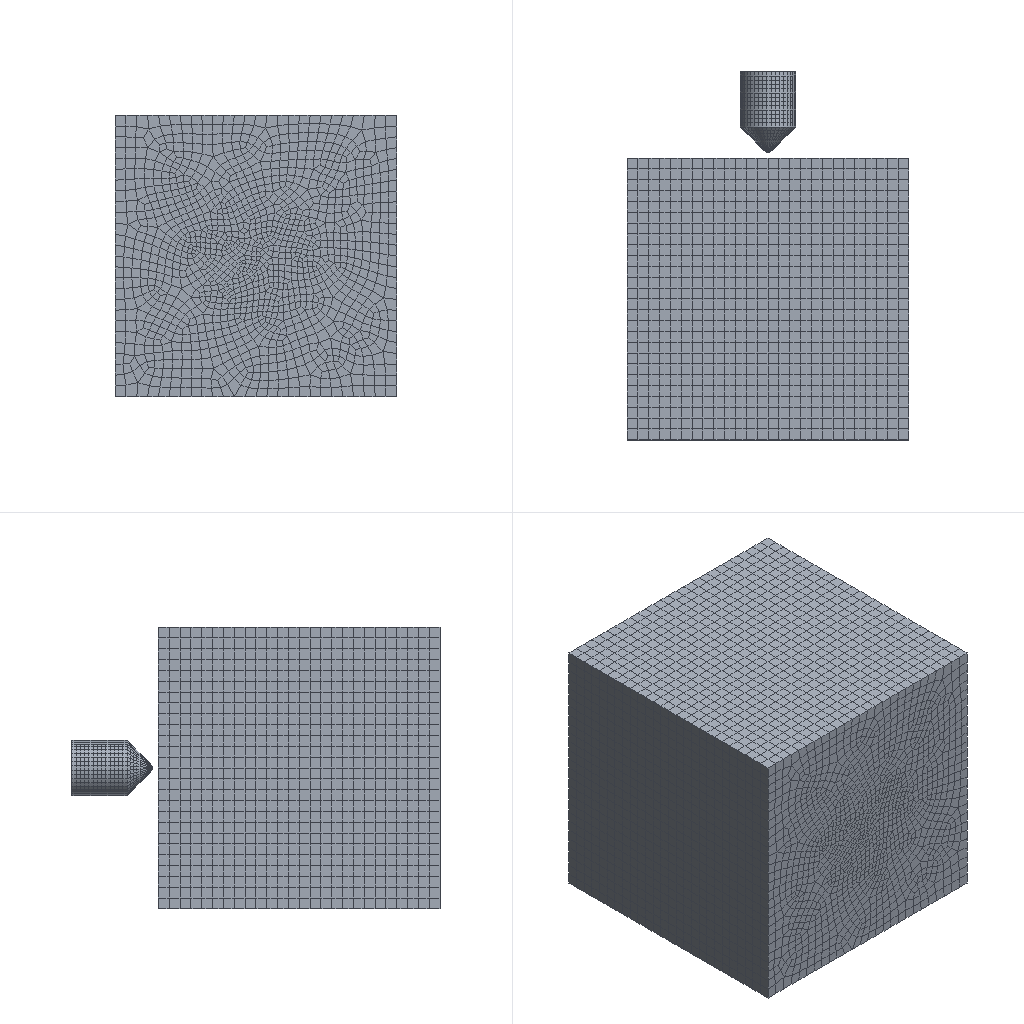Simulation study | abaqus
Set-up summary:
category,name,step,type,value,unit,region
solver,abaqus
solver,version,,,Abaqus/Standard 2020
units,not stated in the deck,,not stated
analysis,deck,,coupled temperature-displacement,coupled temperature-displacement
load_step,Step-1,Step-1,coupled temperature-displacement,nlgeom=True
contact,interactions,,,general=0 pairs=0 ties=1
load_step,requested,,,1
mesh,nodes,,,42891
mesh,elements,,,39512
element_type,C3D6T,,solid,105
element_type,C3D8RT,,solid,39407
load,load commands in deck,,count,2
bc,support commands in deck,,count,3
material,BOLI,,in results
check,setup vs results,,match,"per instance, exact: element labels, types and connectivity; labels of the nodes the elements use; coordinates of those nodes at SINGLE_PRECISION in 2 of 2 instance(s)"
Abaqus input file, long lists of numbers shortened:
*Heading
** Job name: Job-1 Model name: Model-1
** Generated by: Abaqus/CAE 2020
*Preprint, echo=NO, model=NO, history=NO, contact=NO
**
** PARTS
**
*Part, name=Part-1
*Node
      1,   12.396,           0.,   12.396
      2,           0.,           0.,         25.5
** (38797 more lines like these left out)
*Element, type=C3D8RT
    1,    10,     9,     8,   113,  1447,  1446,  1445,  1550
    2,     8,     7,     6,   113,  1445,  1444,  1443,  1550
** (35982 more lines like these left out)
*Nset, nset=Set-1, generate
     1,  38799,      1
*Elset, elset=Set-1, generate
     1,  35984,      1
** Section: boli
*Solid Section, elset=Set-1, material=boli
,
*End Part
**
*Part, name=Part-2
*Node
      1,   2.371,          6.5,  0.7917
      2,   2.214,          6.5,   1.162
** (4090 more lines like these left out)
*Element, type=C3D6T
  1,  307,  302,  298,  121,  116,  112
  2,  359,  291,  285,  173,  105,   99
** (103 more lines like these left out)
*Element, type=C3D8RT
 106,  222,  204,  346,  272,   36,   18,  160,   86
 107,  226,  270,  203,  221,   40,   84,   17,   35
** (3421 more lines like these left out)
*Nset, nset=Set-5, generate
    1,  4092,     1
*Elset, elset=Set-5, generate
    1,  3528,     1
** Section: boli
*Solid Section, elset=Set-5, material=boli
,
*End Part
**
**
** ASSEMBLY
**
*Assembly, name=Assembly
**
*Instance, name=Part-1-1, part=Part-1
*End Instance
**
*Instance, name=Part-2-1, part=Part-2
       12.75,     1.326,        12.75
*End Instance
**
*Nset, nset=Set-1, instance=Part-1-1, generate
 37363,  38799,      1
*Elset, elset=Set-1, instance=Part-1-1, generate
 34601,  35984,      1
*Nset, nset=Set-2, instance=Part-2-1, generate
 3907,  4092,     1
*Elset, elset=Set-2, instance=Part-2-1
  101,  102,  103,  104,  105, 3366, 3367, 3368, 3369, 3370, 3371, 3372, 3373, 3374, 3375, 3376
 3377, 3378, 3379, 3380, 3381, 3382, 3383, 3384, 3385, 3386, 3387, 3388, 3389, 3390, 3391, 3392
** (9 more lines like these left out)
*Nset, nset=Set-3, instance=Part-1-1, generate
     1,  38799,      1
*Nset, nset=Set-3, instance=Part-2-1, generate
    1,  4092,     1
*Elset, elset=Set-3, instance=Part-1-1, generate
     1,  35984,      1
*Elset, elset=Set-3, instance=Part-2-1, generate
    1,  3528,     1
*Nset, nset=Set-4, instance=Part-1-1
   1,   6,   7,   8,   9,  10,  11,  12, 113
*Elset, elset=Set-4, instance=Part-1-1, generate
 1,  4,  1
*Elset, elset=_m_Surf-1_S1, internal, instance=Part-2-1
  101,  102,  103,  104,  105, 3366, 3367, 3368, 3369, 3370, 3371, 3372, 3373, 3374, 3375, 3376
 3377, 3378, 3379, 3380, 3381, 3382, 3383, 3384, 3385, 3386, 3387, 3388, 3389, 3390, 3391, 3392
** (9 more lines like these left out)
*Surface, type=ELEMENT, name=m_Surf-1
_m_Surf-1_S1, S1
*Elset, elset=_s_Surf-1_S1, internal, instance=Part-1-1, generate
    1,  1384,     1
*Surface, type=ELEMENT, name=s_Surf-1
_s_Surf-1_S1, S1
** Constraint: Constraint-1
*Tie, name=Constraint-1, adjust=yes
s_Surf-1, m_Surf-1
*End Assembly
*Amplitude, name=Amp-1
             0.,              0.,              5.,            26.6,             10.,            40.3,             15.,             62.
            20.,            82.3,             25.,           103.5,             30.,            128.,             35.,           147.5
            40.,           166.1,             45.,           182.8,             50.,           197.6,             55.,           206.1
            60.,           209.6,             65.,            213.,             70.,            214.,             75.,            214.
            80.,           216.2,             85.,           216.6,             90.,           216.6,             95.,           218.8
           100.,           219.6,            105.,           216.5,            110.,           214.9,            115.,           214.5
           120.,            215.,            125.,           215.4,            130.,           213.9,            135.,           213.9
           140.,           213.9,            145.,           204.8,            150.,           205.2
**
** MATERIALS
**
*Material, name=boli
*Conductivity
 1.1,
*Density
 2.51e-09,
*Elastic
82000., 0.21
*Expansion
 7.1e-06,
*Specific Heat
 8.79e+08,
**
** PREDEFINED FIELDS
**
** Name: Predefined Field-1   Type: Temperature
*Initial Conditions, type=TEMPERATURE
Set-3, 25.
** ----------------------------------------------------------------
**
** STEP: Step-1
**
*Step, name=Step-1, nlgeom=YES, inc=10000
*Coupled Temperature-displacement, creep=none, deltmx=1e+14, stabilize=0.0002, allsdtol=0.05, continue=NO
0.1, 150., 0.0001, 5.
**
** BOUNDARY CONDITIONS
**
** Name: BC-1 Type: 对称/反对称/完全固定
*Boundary
Set-1, ENCASTRE
** Name: BC-2 Type: 温度
*Boundary, amplitude=Amp-1
Set-2, 11, 11, 1.
** Name: BC-2-Copy Type: 温度
*Boundary, amplitude=Amp-1
Set-4, 11, 11, 1.
**
** OUTPUT REQUESTS
**
*Restart, write, frequency=0
**
** FIELD OUTPUT: F-Output-1
**
*Output, field
*Node Output
CF, NT, RF, RFL, RM, RT, U, V
*Element Output, directions=YES
E, HFL, LE, MISES, MISESMAX, PE, PEEQ, PEMAG, S, SEQUT, TEMP, YIELDPOT
*Contact Output
CDISP, CSTRESS
*Radiation Output
FTEMP,
**
** HISTORY OUTPUT: H-Output-1
**
*Output, history, variable=PRESELECT
*End Step
Results summary:
result,step,,completed,increments=40 time=150.0/150.0
result,analysis,,,"coupled temperature-displacement, steady state"
result,last_loadstep,,,1
result,analysis steps,,count,1
result,primary field,,,"U, NT11"
result,reaction total,,FX,-0.000189,model units
result,reaction total,,FY,0.402,model units
result,reaction total,,FZ,0.00182,model units